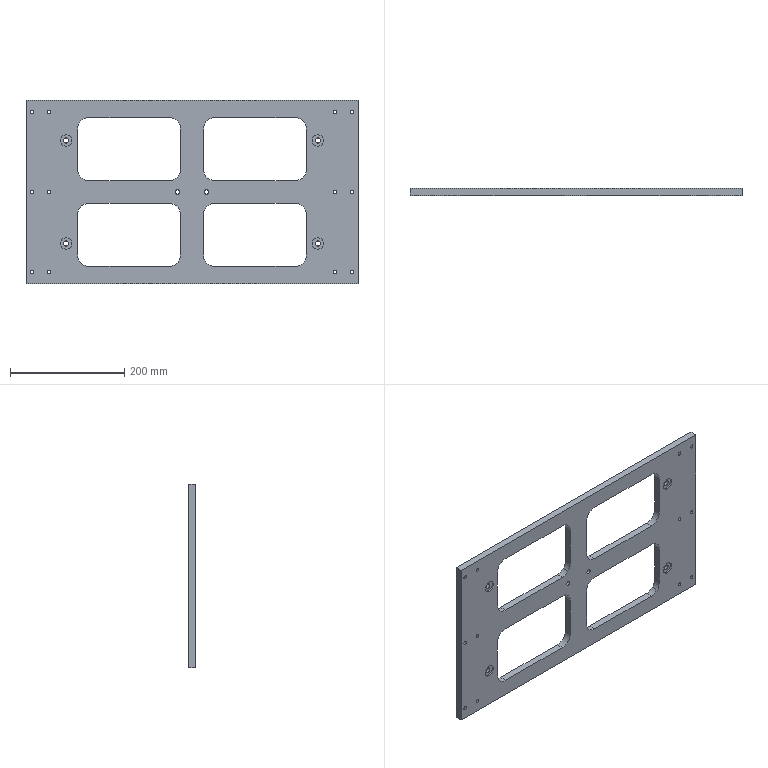Part | STEP file | PUSH.PLATE.stp | 1 solid | 94 faces | box 580 x 12 x 320 mm | volume 1281951 mm3 | cylinder 40 | spline 40 | plane 14 | commonest cylinder face diameters 40 x16 6 x12 8 x4 9 x4 20 x4